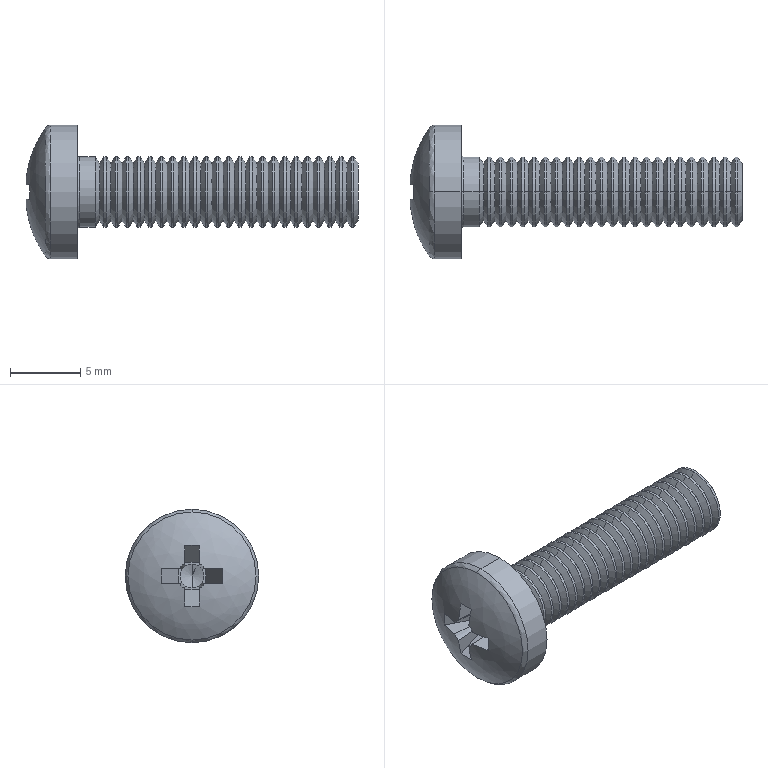Part | SolidWorks | features BaseBody 1 | 1 solid | 173 faces | box 23.632 x 9.5 x 9.5 mm | volume 537.774 mm3 | cone 100 | cylinder 50 | plane 18 | spline 5 | commonest cylinder face diameters 5 x48 9.5 x2